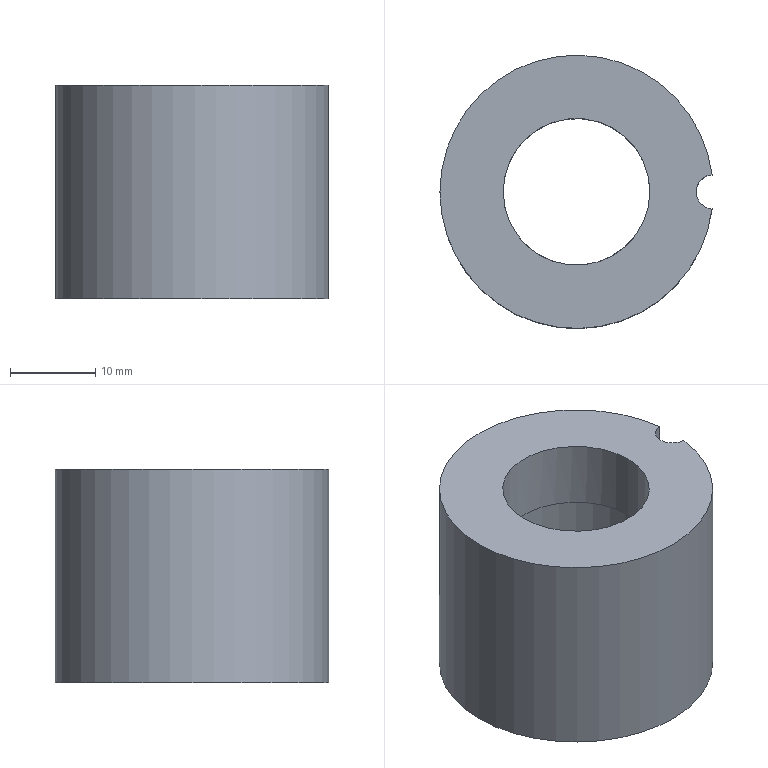Part | NX | features solid 2 | 1 solid | 7 faces | box 31.875 x 32 x 25 mm | volume 12433 mm3 | cylinder 4 | plane 3 | commonest cylinder face diameters 4 x1 17.18 x1 20.6 x1 32 x1
STEP:
#1=CARTESIAN_POINT('',(-505.667,-135.826,-12.395));
#2=VERTEX_POINT('',#1);
#3=CARTESIAN_POINT('',(-505.667,-139.818,-12.395));
#4=VERTEX_POINT('',#3);
#5=CARTESIAN_POINT('',(-505.542,-137.822,-12.395));
#6=DIRECTION('',(0.,0.,1.));
#7=DIRECTION('',(1.,0.,0.));
#8=AXIS2_PLACEMENT_3D('',#5,#6,#7);
#9=CIRCLE('',#8,2.);
#10=EDGE_CURVE('',#2,#4,#9,.T.);
#11=ORIENTED_EDGE('',*,*,#10,.F.);
#12=CARTESIAN_POINT('',(-521.542,-137.822,-12.395));
#13=DIRECTION('',(0.,0.,-1.));
#14=DIRECTION('',(-1.,0.,0.));
#15=AXIS2_PLACEMENT_3D('',#12,#13,#14);
#16=CIRCLE('',#15,16.);
#17=EDGE_CURVE('',#4,#2,#16,.T.);
#18=ORIENTED_EDGE('',*,*,#17,.F.);
#19=EDGE_LOOP('',(#11,#18));
#20=FACE_BOUND('',#19,.T.);
#21=CARTESIAN_POINT('',(-530.132,-137.822,-12.395));
#22=VERTEX_POINT('',#21);
#23=CARTESIAN_POINT('',(-521.542,-137.822,-12.395));
#24=DIRECTION('',(0.,0.,-1.));
#25=DIRECTION('',(-1.,0.,0.));
#26=AXIS2_PLACEMENT_3D('',#23,#24,#25);
#27=CIRCLE('',#26,8.59);
#28=EDGE_CURVE('',#22,#22,#27,.T.);
#29=ORIENTED_EDGE('',*,*,#28,.T.);
#30=EDGE_LOOP('',(#29));
#31=FACE_BOUND('',#30,.T.);
#32=CARTESIAN_POINT('',(-521.542,-137.822,-12.395));
#33=DIRECTION('',(0.,0.,1.));
#34=DIRECTION('',(1.,0.,0.));
#35=AXIS2_PLACEMENT_3D('',#32,#33,#34);
#36=PLANE('',#35);
#37=ADVANCED_FACE('',(#20,#31),#36,.T.);
#38=CARTESIAN_POINT('',(-505.667,-135.826,-37.395));
#39=VERTEX_POINT('',#38);
#40=CARTESIAN_POINT('',(-505.667,-139.818,-37.395));
#41=VERTEX_POINT('',#40);
#42=CARTESIAN_POINT('',(-505.542,-137.822,-37.395));
#43=DIRECTION('',(0.,0.,1.));
#44=DIRECTION('',(1.,0.,0.));
#45=AXIS2_PLACEMENT_3D('',#42,#43,#44);
#46=CIRCLE('',#45,2.);
#47=EDGE_CURVE('',#39,#41,#46,.T.);
#48=ORIENTED_EDGE('',*,*,#47,.T.);
#49=CARTESIAN_POINT('',(-521.542,-137.822,-37.395));
#50=DIRECTION('',(0.,0.,1.));
#51=DIRECTION('',(1.,0.,0.));
#52=AXIS2_PLACEMENT_3D('',#49,#50,#51);
#53=CIRCLE('',#52,16.);
#54=EDGE_CURVE('',#39,#41,#53,.T.);
#55=ORIENTED_EDGE('',*,*,#54,.F.);
#56=EDGE_LOOP('',(#48,#55));
#57=FACE_BOUND('',#56,.T.);
#58=CARTESIAN_POINT('',(-511.242,-137.822,-37.395));
#59=VERTEX_POINT('',#58);
#60=CARTESIAN_POINT('',(-521.542,-137.822,-37.395));
#61=DIRECTION('',(0.,0.,1.));
#62=DIRECTION('',(1.,0.,0.));
#63=AXIS2_PLACEMENT_3D('',#60,#61,#62);
#64=CIRCLE('',#63,10.3);
#65=EDGE_CURVE('',#59,#59,#64,.T.);
#66=ORIENTED_EDGE('',*,*,#65,.T.);
#67=EDGE_LOOP('',(#66));
#68=FACE_BOUND('',#67,.T.);
#69=CARTESIAN_POINT('',(-521.542,-137.822,-37.395));
#70=DIRECTION('',(0.,0.,-1.));
#71=DIRECTION('',(-1.,0.,0.));
#72=AXIS2_PLACEMENT_3D('',#69,#70,#71);
#73=PLANE('',#72);
#74=ADVANCED_FACE('',(#57,#68),#73,.T.);
#75=CARTESIAN_POINT('',(-505.667,-135.826,-24.895));
#76=DIRECTION('',(0.,0.,1.));
#77=VECTOR('',#76,1000.);
#78=LINE('',#75,#77);
#79=EDGE_CURVE('',#39,#2,#78,.T.);
#80=ORIENTED_EDGE('',*,*,#79,.F.);
#81=ORIENTED_EDGE('',*,*,#54,.T.);
#82=CARTESIAN_POINT('',(-505.667,-139.818,-24.895));
#83=DIRECTION('',(0.,0.,1.));
#84=VECTOR('',#83,1000.);
#85=LINE('',#82,#84);
#86=EDGE_CURVE('',#4,#41,#85,.F.);
#87=ORIENTED_EDGE('',*,*,#86,.F.);
#88=ORIENTED_EDGE('',*,*,#17,.T.);
#89=EDGE_LOOP('',(#80,#81,#87,#88));
#90=FACE_BOUND('',#89,.T.);
#91=CARTESIAN_POINT('',(-521.542,-137.822,-37.395));
#92=DIRECTION('',(0.,0.,1.));
#93=DIRECTION('',(1.,0.,0.));
#94=AXIS2_PLACEMENT_3D('',#91,#92,#93);
#95=CYLINDRICAL_SURFACE('',#94,16.);
#96=ADVANCED_FACE('',(#90),#95,.T.);
#97=CARTESIAN_POINT('',(-512.952,-137.822,-20.395));
#98=VERTEX_POINT('',#97);
#99=CARTESIAN_POINT('',(-521.542,-137.822,-20.395));
#100=DIRECTION('',(0.,0.,1.));
#101=DIRECTION('',(1.,0.,0.));
#102=AXIS2_PLACEMENT_3D('',#99,#100,#101);
#103=CIRCLE('',#102,8.59);
#104=EDGE_CURVE('',#98,#98,#103,.T.);
#105=ORIENTED_EDGE('',*,*,#104,.T.);
#106=EDGE_LOOP('',(#105));
#107=FACE_BOUND('',#106,.T.);
#108=CARTESIAN_POINT('',(-531.842,-137.822,-20.395));
#109=VERTEX_POINT('',#108);
#110=CARTESIAN_POINT('',(-521.542,-137.822,-20.395));
#111=DIRECTION('',(0.,0.,-1.));
#112=DIRECTION('',(-1.,0.,0.));
#113=AXIS2_PLACEMENT_3D('',#110,#111,#112);
#114=CIRCLE('',#113,10.3);
#115=EDGE_CURVE('',#109,#109,#114,.T.);
#116=ORIENTED_EDGE('',*,*,#115,.T.);
#117=EDGE_LOOP('',(#116));
#118=FACE_BOUND('',#117,.T.);
#119=CARTESIAN_POINT('',(-521.542,-137.822,-20.395));
#120=DIRECTION('',(0.,0.,1.));
#121=DIRECTION('',(1.,0.,0.));
#122=AXIS2_PLACEMENT_3D('',#119,#120,#121);
#123=PLANE('',#122);
#124=ADVANCED_FACE('',(#107,#118),#123,.F.);
#125=ORIENTED_EDGE('',*,*,#115,.F.);
#126=EDGE_LOOP('',(#125));
#127=FACE_BOUND('',#126,.T.);
#128=ORIENTED_EDGE('',*,*,#65,.F.);
#129=EDGE_LOOP('',(#128));
#130=FACE_BOUND('',#129,.T.);
#131=CARTESIAN_POINT('',(-521.542,-137.822,-37.395));
#132=DIRECTION('',(0.,0.,1.));
#133=DIRECTION('',(1.,0.,0.));
#134=AXIS2_PLACEMENT_3D('',#131,#132,#133);
#135=CYLINDRICAL_SURFACE('',#134,10.3);
#136=ADVANCED_FACE('',(#127,#130),#135,.F.);
#137=ORIENTED_EDGE('',*,*,#28,.F.);
#138=EDGE_LOOP('',(#137));
#139=FACE_BOUND('',#138,.T.);
#140=ORIENTED_EDGE('',*,*,#104,.F.);
#141=EDGE_LOOP('',(#140));
#142=FACE_BOUND('',#141,.T.);
#143=CARTESIAN_POINT('',(-521.542,-137.822,-20.395));
#144=DIRECTION('',(0.,0.,1.));
#145=DIRECTION('',(1.,0.,0.));
#146=AXIS2_PLACEMENT_3D('',#143,#144,#145);
#147=CYLINDRICAL_SURFACE('',#146,8.59);
#148=ADVANCED_FACE('',(#139,#142),#147,.F.);
#149=ORIENTED_EDGE('',*,*,#79,.T.);
#150=ORIENTED_EDGE('',*,*,#10,.T.);
#151=ORIENTED_EDGE('',*,*,#86,.T.);
#152=ORIENTED_EDGE('',*,*,#47,.F.);
#153=EDGE_LOOP('',(#149,#150,#151,#152));
#154=FACE_BOUND('',#153,.T.);
#155=CARTESIAN_POINT('',(-505.542,-137.822,-37.395));
#156=DIRECTION('',(0.,0.,1.));
#157=DIRECTION('',(1.,0.,0.));
#158=AXIS2_PLACEMENT_3D('',#155,#156,#157);
#159=CYLINDRICAL_SURFACE('',#158,2.);
#160=ADVANCED_FACE('',(#154),#159,.F.);
#161=CLOSED_SHELL('',(#37,#74,#96,#124,#136,#148,#160));
#162=MANIFOLD_SOLID_BREP('',#161);
#163=(LENGTH_UNIT()NAMED_UNIT(*)SI_UNIT(.MILLI.,.METRE.));
#164=UNCERTAINTY_MEASURE_WITH_UNIT(LENGTH_MEASURE(0.00001),#163,'','');
#165=(NAMED_UNIT(*)PLANE_ANGLE_UNIT()SI_UNIT($,.RADIAN.));
#166=(NAMED_UNIT(*)SI_UNIT($,.STERADIAN.)SOLID_ANGLE_UNIT());
#167=(GEOMETRIC_REPRESENTATION_CONTEXT(3)GLOBAL_UNCERTAINTY_ASSIGNED_CONTEXT((#164))GLOBAL_UNIT_ASSIGNED_CONTEXT((#163,#165,#166))REPRESENTATION_CONTEXT('',''));
#168=ADVANCED_BREP_SHAPE_REPRESENTATION('',(#162),#167);